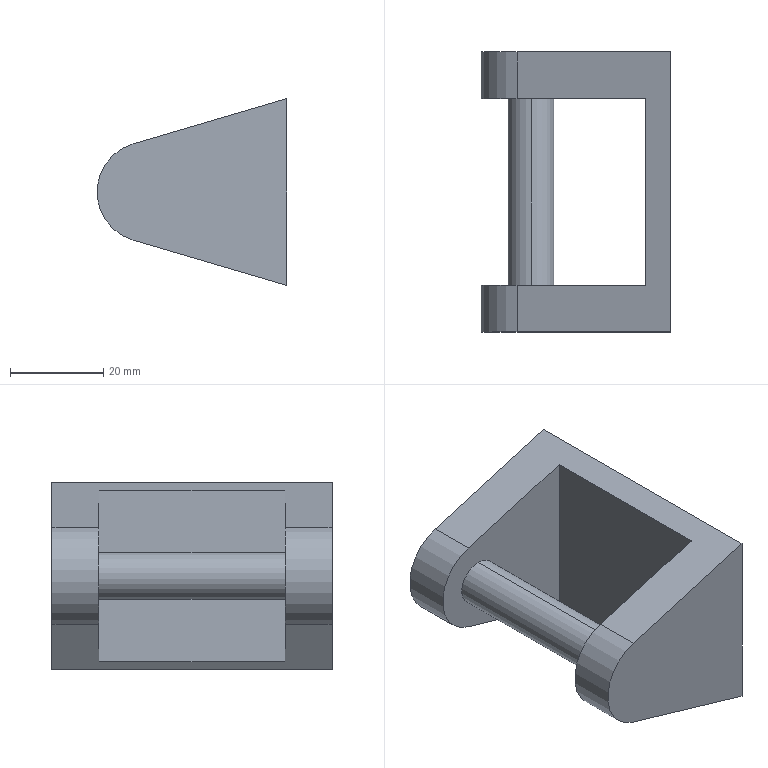Part | SolidWorks | features ICE 2, Extrusion 1 | 1 solid | 12 faces | box 40.645 x 60 x 40 mm | volume 33727 mm3 | plane 8 | cylinder 4 | commonest cylinder face diameters 10 x2 21.526 x2
STEP:
#1=CARTESIAN_POINT('',(-29.882,50.,15.));
#2=VERTEX_POINT('',#1);
#3=CARTESIAN_POINT('',(-29.882,50.,25.));
#4=VERTEX_POINT('',#3);
#5=CARTESIAN_POINT('',(-29.882,50.,20.));
#6=DIRECTION('',(0.,-1.,0.));
#7=DIRECTION('',(0.,0.,-1.));
#8=AXIS2_PLACEMENT_3D('',#5,#6,#7);
#9=CIRCLE('',#8,5.);
#10=EDGE_CURVE('',#2,#4,#9,.T.);
#11=ORIENTED_EDGE('',*,*,#10,.T.);
#12=CARTESIAN_POINT('',(-29.882,10.,25.));
#13=VERTEX_POINT('',#12);
#14=CARTESIAN_POINT('',(-29.882,60.002,25.));
#15=DIRECTION('',(0.,-1.,0.));
#16=VECTOR('',#15,1000.);
#17=LINE('',#14,#16);
#18=EDGE_CURVE('',#4,#13,#17,.T.);
#19=ORIENTED_EDGE('',*,*,#18,.T.);
#20=CARTESIAN_POINT('',(-29.882,10.,15.));
#21=VERTEX_POINT('',#20);
#22=CARTESIAN_POINT('',(-29.882,10.,20.));
#23=DIRECTION('',(0.,-1.,0.));
#24=DIRECTION('',(0.,0.,-1.));
#25=AXIS2_PLACEMENT_3D('',#22,#23,#24);
#26=CIRCLE('',#25,5.);
#27=EDGE_CURVE('',#21,#13,#26,.T.);
#28=ORIENTED_EDGE('',*,*,#27,.F.);
#29=CARTESIAN_POINT('',(-29.882,60.002,15.));
#30=DIRECTION('',(0.,-1.,0.));
#31=VECTOR('',#30,1000.);
#32=LINE('',#29,#31);
#33=EDGE_CURVE('',#2,#21,#32,.T.);
#34=ORIENTED_EDGE('',*,*,#33,.F.);
#35=EDGE_LOOP('',(#11,#19,#28,#34));
#36=FACE_OUTER_BOUND('',#35,.T.);
#37=CARTESIAN_POINT('',(-29.882,60.002,20.));
#38=DIRECTION('',(0.,-1.,0.));
#39=DIRECTION('',(0.,0.,-1.));
#40=AXIS2_PLACEMENT_3D('',#37,#38,#39);
#41=CYLINDRICAL_SURFACE('',#40,5.);
#42=ADVANCED_FACE('',(#36),#41,.T.);
#43=CARTESIAN_POINT('',(-32.917,50.,9.673));
#44=VERTEX_POINT('',#43);
#45=CARTESIAN_POINT('',(-5.382,50.,1.581));
#46=VERTEX_POINT('',#45);
#47=CARTESIAN_POINT('',(-32.917,50.,9.673));
#48=DIRECTION('',(0.9594,0.,-0.282));
#49=VECTOR('',#48,1000.);
#50=LINE('',#47,#49);
#51=EDGE_CURVE('',#44,#46,#50,.T.);
#52=ORIENTED_EDGE('',*,*,#51,.F.);
#53=CARTESIAN_POINT('',(-32.917,60.,9.673));
#54=VERTEX_POINT('',#53);
#55=CARTESIAN_POINT('',(-32.917,60.,9.673));
#56=DIRECTION('',(0.,-1.,0.));
#57=VECTOR('',#56,1000.);
#58=LINE('',#55,#57);
#59=EDGE_CURVE('',#54,#44,#58,.T.);
#60=ORIENTED_EDGE('',*,*,#59,.F.);
#61=CARTESIAN_POINT('',(0.,60.,0.));
#62=VERTEX_POINT('',#61);
#63=CARTESIAN_POINT('',(0.,60.,0.));
#64=DIRECTION('',(-0.9594,0.,0.282));
#65=VECTOR('',#64,1000.);
#66=LINE('',#63,#65);
#67=EDGE_CURVE('',#62,#54,#66,.T.);
#68=ORIENTED_EDGE('',*,*,#67,.F.);
#69=CARTESIAN_POINT('',(0.,0.,0.));
#70=VERTEX_POINT('',#69);
#71=CARTESIAN_POINT('',(0.,60.,0.));
#72=DIRECTION('',(0.,-1.,0.));
#73=VECTOR('',#72,1000.);
#74=LINE('',#71,#73);
#75=EDGE_CURVE('',#62,#70,#74,.T.);
#76=ORIENTED_EDGE('',*,*,#75,.T.);
#77=CARTESIAN_POINT('',(-32.917,0.,9.673));
#78=VERTEX_POINT('',#77);
#79=CARTESIAN_POINT('',(0.,0.,0.));
#80=DIRECTION('',(-0.9594,0.,0.282));
#81=VECTOR('',#80,1000.);
#82=LINE('',#79,#81);
#83=EDGE_CURVE('',#70,#78,#82,.T.);
#84=ORIENTED_EDGE('',*,*,#83,.T.);
#85=CARTESIAN_POINT('',(-32.917,10.,9.673));
#86=VERTEX_POINT('',#85);
#87=CARTESIAN_POINT('',(-32.917,60.,9.673));
#88=DIRECTION('',(0.,-1.,0.));
#89=VECTOR('',#88,1000.);
#90=LINE('',#87,#89);
#91=EDGE_CURVE('',#86,#78,#90,.T.);
#92=ORIENTED_EDGE('',*,*,#91,.F.);
#93=CARTESIAN_POINT('',(-5.382,10.,1.581));
#94=VERTEX_POINT('',#93);
#95=CARTESIAN_POINT('',(-32.917,10.,9.673));
#96=DIRECTION('',(0.9594,0.,-0.282));
#97=VECTOR('',#96,1000.);
#98=LINE('',#95,#97);
#99=EDGE_CURVE('',#86,#94,#98,.T.);
#100=ORIENTED_EDGE('',*,*,#99,.T.);
#101=CARTESIAN_POINT('',(-5.382,50.,1.581));
#102=DIRECTION('',(0.,-1.,0.));
#103=VECTOR('',#102,1000.);
#104=LINE('',#101,#103);
#105=EDGE_CURVE('',#46,#94,#104,.T.);
#106=ORIENTED_EDGE('',*,*,#105,.F.);
#107=EDGE_LOOP('',(#52,#60,#68,#76,#84,#92,#100,#106));
#108=FACE_OUTER_BOUND('',#107,.T.);
#109=CARTESIAN_POINT('',(0.,60.,0.));
#110=DIRECTION('',(0.282,0.,0.9594));
#111=DIRECTION('',(0.9594,0.,-0.282));
#112=AXIS2_PLACEMENT_3D('',#109,#110,#111);
#113=PLANE('',#112);
#114=ADVANCED_FACE('',(#108),#113,.F.);
#115=CARTESIAN_POINT('',(-32.917,50.,30.327));
#116=VERTEX_POINT('',#115);
#117=CARTESIAN_POINT('',(-29.882,50.,20.));
#118=DIRECTION('',(0.,-1.,0.));
#119=DIRECTION('',(0.,0.,-1.));
#120=AXIS2_PLACEMENT_3D('',#117,#118,#119);
#121=CIRCLE('',#120,10.763);
#122=EDGE_CURVE('',#116,#44,#121,.T.);
#123=ORIENTED_EDGE('',*,*,#122,.F.);
#124=CARTESIAN_POINT('',(-32.917,60.,30.327));
#125=VERTEX_POINT('',#124);
#126=CARTESIAN_POINT('',(-32.917,60.,30.327));
#127=DIRECTION('',(0.,-1.,0.));
#128=VECTOR('',#127,1000.);
#129=LINE('',#126,#128);
#130=EDGE_CURVE('',#125,#116,#129,.T.);
#131=ORIENTED_EDGE('',*,*,#130,.F.);
#132=CARTESIAN_POINT('',(-29.882,60.,20.));
#133=DIRECTION('',(0.,1.,0.));
#134=DIRECTION('',(0.,0.,-1.));
#135=AXIS2_PLACEMENT_3D('',#132,#133,#134);
#136=CIRCLE('',#135,10.763);
#137=EDGE_CURVE('',#54,#125,#136,.T.);
#138=ORIENTED_EDGE('',*,*,#137,.F.);
#139=ORIENTED_EDGE('',*,*,#59,.T.);
#140=EDGE_LOOP('',(#123,#131,#138,#139));
#141=FACE_OUTER_BOUND('',#140,.T.);
#142=CARTESIAN_POINT('',(-29.882,60.,20.));
#143=DIRECTION('',(0.,-1.,0.));
#144=DIRECTION('',(0.,0.,-1.));
#145=AXIS2_PLACEMENT_3D('',#142,#143,#144);
#146=CYLINDRICAL_SURFACE('',#145,10.763);
#147=ADVANCED_FACE('',(#141),#146,.T.);
#148=CARTESIAN_POINT('',(-5.382,50.,38.419));
#149=VERTEX_POINT('',#148);
#150=CARTESIAN_POINT('',(-5.382,50.,38.419));
#151=DIRECTION('',(-0.9594,0.,-0.282));
#152=VECTOR('',#151,1000.);
#153=LINE('',#150,#152);
#154=EDGE_CURVE('',#149,#116,#153,.T.);
#155=ORIENTED_EDGE('',*,*,#154,.F.);
#156=CARTESIAN_POINT('',(-5.382,10.,38.419));
#157=VERTEX_POINT('',#156);
#158=CARTESIAN_POINT('',(-5.382,50.,38.419));
#159=DIRECTION('',(0.,-1.,0.));
#160=VECTOR('',#159,1000.);
#161=LINE('',#158,#160);
#162=EDGE_CURVE('',#149,#157,#161,.T.);
#163=ORIENTED_EDGE('',*,*,#162,.T.);
#164=CARTESIAN_POINT('',(-32.917,10.,30.327));
#165=VERTEX_POINT('',#164);
#166=CARTESIAN_POINT('',(-5.382,10.,38.419));
#167=DIRECTION('',(-0.9594,0.,-0.282));
#168=VECTOR('',#167,1000.);
#169=LINE('',#166,#168);
#170=EDGE_CURVE('',#157,#165,#169,.T.);
#171=ORIENTED_EDGE('',*,*,#170,.T.);
#172=CARTESIAN_POINT('',(-32.917,0.,30.327));
#173=VERTEX_POINT('',#172);
#174=CARTESIAN_POINT('',(-32.917,60.,30.327));
#175=DIRECTION('',(0.,-1.,0.));
#176=VECTOR('',#175,1000.);
#177=LINE('',#174,#176);
#178=EDGE_CURVE('',#165,#173,#177,.T.);
#179=ORIENTED_EDGE('',*,*,#178,.T.);
#180=CARTESIAN_POINT('',(0.,0.,40.));
#181=VERTEX_POINT('',#180);
#182=CARTESIAN_POINT('',(0.,0.,40.));
#183=DIRECTION('',(0.9594,0.,0.282));
#184=VECTOR('',#183,1000.);
#185=LINE('',#182,#184);
#186=EDGE_CURVE('',#173,#181,#185,.T.);
#187=ORIENTED_EDGE('',*,*,#186,.T.);
#188=CARTESIAN_POINT('',(0.,60.,40.));
#189=VERTEX_POINT('',#188);
#190=CARTESIAN_POINT('',(0.,60.,40.));
#191=DIRECTION('',(0.,-1.,0.));
#192=VECTOR('',#191,1000.);
#193=LINE('',#190,#192);
#194=EDGE_CURVE('',#189,#181,#193,.T.);
#195=ORIENTED_EDGE('',*,*,#194,.F.);
#196=CARTESIAN_POINT('',(0.,60.,40.));
#197=DIRECTION('',(0.9594,0.,0.282));
#198=VECTOR('',#197,1000.);
#199=LINE('',#196,#198);
#200=EDGE_CURVE('',#125,#189,#199,.T.);
#201=ORIENTED_EDGE('',*,*,#200,.F.);
#202=ORIENTED_EDGE('',*,*,#130,.T.);
#203=EDGE_LOOP('',(#155,#163,#171,#179,#187,#195,#201,#202));
#204=FACE_OUTER_BOUND('',#203,.T.);
#205=CARTESIAN_POINT('',(0.,60.,40.));
#206=DIRECTION('',(0.282,0.,-0.9594));
#207=DIRECTION('',(-0.9594,0.,-0.282));
#208=AXIS2_PLACEMENT_3D('',#205,#206,#207);
#209=PLANE('',#208);
#210=ADVANCED_FACE('',(#204),#209,.F.);
#211=ORIENTED_EDGE('',*,*,#178,.F.);
#212=CARTESIAN_POINT('',(-29.882,10.,20.));
#213=DIRECTION('',(0.,-1.,0.));
#214=DIRECTION('',(0.,0.,-1.));
#215=AXIS2_PLACEMENT_3D('',#212,#213,#214);
#216=CIRCLE('',#215,10.763);
#217=EDGE_CURVE('',#165,#86,#216,.T.);
#218=ORIENTED_EDGE('',*,*,#217,.T.);
#219=ORIENTED_EDGE('',*,*,#91,.T.);
#220=CARTESIAN_POINT('',(-29.882,0.,20.));
#221=DIRECTION('',(0.,1.,0.));
#222=DIRECTION('',(0.,0.,-1.));
#223=AXIS2_PLACEMENT_3D('',#220,#221,#222);
#224=CIRCLE('',#223,10.763);
#225=EDGE_CURVE('',#78,#173,#224,.T.);
#226=ORIENTED_EDGE('',*,*,#225,.T.);
#227=EDGE_LOOP('',(#211,#218,#219,#226));
#228=FACE_OUTER_BOUND('',#227,.T.);
#229=CARTESIAN_POINT('',(-29.882,60.,20.));
#230=DIRECTION('',(0.,-1.,0.));
#231=DIRECTION('',(0.,0.,-1.));
#232=AXIS2_PLACEMENT_3D('',#229,#230,#231);
#233=CYLINDRICAL_SURFACE('',#232,10.763);
#234=ADVANCED_FACE('',(#228),#233,.T.);
#235=CARTESIAN_POINT('',(0.,0.,0.));
#236=DIRECTION('',(0.,0.,-1.));
#237=VECTOR('',#236,1000.);
#238=LINE('',#235,#237);
#239=EDGE_CURVE('',#181,#70,#238,.T.);
#240=ORIENTED_EDGE('',*,*,#239,.T.);
#241=ORIENTED_EDGE('',*,*,#75,.F.);
#242=CARTESIAN_POINT('',(0.,60.,0.));
#243=DIRECTION('',(0.,0.,-1.));
#244=VECTOR('',#243,1000.);
#245=LINE('',#242,#244);
#246=EDGE_CURVE('',#189,#62,#245,.T.);
#247=ORIENTED_EDGE('',*,*,#246,.F.);
#248=ORIENTED_EDGE('',*,*,#194,.T.);
#249=EDGE_LOOP('',(#240,#241,#247,#248));
#250=FACE_OUTER_BOUND('',#249,.T.);
#251=CARTESIAN_POINT('',(0.,60.,0.));
#252=DIRECTION('',(-1.,0.,0.));
#253=DIRECTION('',(0.,0.,1.));
#254=AXIS2_PLACEMENT_3D('',#251,#252,#253);
#255=PLANE('',#254);
#256=ADVANCED_FACE('',(#250),#255,.F.);
#257=ORIENTED_EDGE('',*,*,#67,.T.);
#258=ORIENTED_EDGE('',*,*,#137,.T.);
#259=ORIENTED_EDGE('',*,*,#200,.T.);
#260=ORIENTED_EDGE('',*,*,#246,.T.);
#261=EDGE_LOOP('',(#257,#258,#259,#260));
#262=FACE_OUTER_BOUND('',#261,.T.);
#263=CARTESIAN_POINT('',(-29.882,60.,20.));
#264=DIRECTION('',(0.,-1.,0.));
#265=DIRECTION('',(0.,0.,-1.));
#266=AXIS2_PLACEMENT_3D('',#263,#264,#265);
#267=PLANE('',#266);
#268=ADVANCED_FACE('',(#262),#267,.F.);
#269=ORIENTED_EDGE('',*,*,#83,.F.);
#270=ORIENTED_EDGE('',*,*,#239,.F.);
#271=ORIENTED_EDGE('',*,*,#186,.F.);
#272=ORIENTED_EDGE('',*,*,#225,.F.);
#273=EDGE_LOOP('',(#269,#270,#271,#272));
#274=FACE_OUTER_BOUND('',#273,.T.);
#275=CARTESIAN_POINT('',(-29.882,0.,20.));
#276=DIRECTION('',(0.,-1.,0.));
#277=DIRECTION('',(0.,0.,-1.));
#278=AXIS2_PLACEMENT_3D('',#275,#276,#277);
#279=PLANE('',#278);
#280=ADVANCED_FACE('',(#274),#279,.T.);
#281=CARTESIAN_POINT('',(-5.382,10.,1.581));
#282=DIRECTION('',(0.,0.,1.));
#283=VECTOR('',#282,1000.);
#284=LINE('',#281,#283);
#285=EDGE_CURVE('',#94,#157,#284,.T.);
#286=ORIENTED_EDGE('',*,*,#285,.T.);
#287=ORIENTED_EDGE('',*,*,#162,.F.);
#288=CARTESIAN_POINT('',(-5.382,50.,1.581));
#289=DIRECTION('',(0.,0.,1.));
#290=VECTOR('',#289,1000.);
#291=LINE('',#288,#290);
#292=EDGE_CURVE('',#46,#149,#291,.T.);
#293=ORIENTED_EDGE('',*,*,#292,.F.);
#294=ORIENTED_EDGE('',*,*,#105,.T.);
#295=EDGE_LOOP('',(#286,#287,#293,#294));
#296=FACE_OUTER_BOUND('',#295,.T.);
#297=CARTESIAN_POINT('',(-5.382,50.,1.581));
#298=DIRECTION('',(1.,0.,0.));
#299=DIRECTION('',(0.,0.,-1.));
#300=AXIS2_PLACEMENT_3D('',#297,#298,#299);
#301=PLANE('',#300);
#302=ADVANCED_FACE('',(#296),#301,.F.);
#303=ORIENTED_EDGE('',*,*,#10,.F.);
#304=CARTESIAN_POINT('',(-29.882,50.,20.));
#305=DIRECTION('',(0.,-1.,0.));
#306=DIRECTION('',(0.,0.,-1.));
#307=AXIS2_PLACEMENT_3D('',#304,#305,#306);
#308=CIRCLE('',#307,5.);
#309=EDGE_CURVE('',#4,#2,#308,.T.);
#310=ORIENTED_EDGE('',*,*,#309,.F.);
#311=EDGE_LOOP('',(#303,#310));
#312=FACE_BOUND('',#311,.T.);
#313=ORIENTED_EDGE('',*,*,#51,.T.);
#314=ORIENTED_EDGE('',*,*,#292,.T.);
#315=ORIENTED_EDGE('',*,*,#154,.T.);
#316=ORIENTED_EDGE('',*,*,#122,.T.);
#317=EDGE_LOOP('',(#313,#314,#315,#316));
#318=FACE_OUTER_BOUND('',#317,.T.);
#319=CARTESIAN_POINT('',(-29.882,50.,20.));
#320=DIRECTION('',(0.,-1.,0.));
#321=DIRECTION('',(0.,0.,-1.));
#322=AXIS2_PLACEMENT_3D('',#319,#320,#321);
#323=PLANE('',#322);
#324=ADVANCED_FACE('',(#312,#318),#323,.T.);
#325=ORIENTED_EDGE('',*,*,#27,.T.);
#326=CARTESIAN_POINT('',(-29.882,10.,20.));
#327=DIRECTION('',(0.,-1.,0.));
#328=DIRECTION('',(0.,0.,-1.));
#329=AXIS2_PLACEMENT_3D('',#326,#327,#328);
#330=CIRCLE('',#329,5.);
#331=EDGE_CURVE('',#13,#21,#330,.T.);
#332=ORIENTED_EDGE('',*,*,#331,.T.);
#333=EDGE_LOOP('',(#325,#332));
#334=FACE_BOUND('',#333,.T.);
#335=ORIENTED_EDGE('',*,*,#99,.F.);
#336=ORIENTED_EDGE('',*,*,#217,.F.);
#337=ORIENTED_EDGE('',*,*,#170,.F.);
#338=ORIENTED_EDGE('',*,*,#285,.F.);
#339=EDGE_LOOP('',(#335,#336,#337,#338));
#340=FACE_OUTER_BOUND('',#339,.T.);
#341=CARTESIAN_POINT('',(-29.882,10.,20.));
#342=DIRECTION('',(0.,-1.,0.));
#343=DIRECTION('',(0.,0.,-1.));
#344=AXIS2_PLACEMENT_3D('',#341,#342,#343);
#345=PLANE('',#344);
#346=ADVANCED_FACE('',(#334,#340),#345,.F.);
#347=ORIENTED_EDGE('',*,*,#18,.F.);
#348=ORIENTED_EDGE('',*,*,#309,.T.);
#349=ORIENTED_EDGE('',*,*,#33,.T.);
#350=ORIENTED_EDGE('',*,*,#331,.F.);
#351=EDGE_LOOP('',(#347,#348,#349,#350));
#352=FACE_OUTER_BOUND('',#351,.T.);
#353=CARTESIAN_POINT('',(-29.882,60.002,20.));
#354=DIRECTION('',(0.,-1.,0.));
#355=DIRECTION('',(0.,0.,-1.));
#356=AXIS2_PLACEMENT_3D('',#353,#354,#355);
#357=CYLINDRICAL_SURFACE('',#356,5.);
#358=ADVANCED_FACE('',(#352),#357,.T.);
#359=CLOSED_SHELL('',(#42,#114,#147,#210,#234,#256,#268,#280,#302,#324,#346,#358));
#360=MANIFOLD_SOLID_BREP('',#359);
#361=CARTESIAN_POINT('',(0.,0.,0.));
#362=DIRECTION('',(0.,0.,1.));
#363=DIRECTION('',(1.,0.,0.));
#364=AXIS2_PLACEMENT_3D('',#361,#362,#363);
#365=(LENGTH_UNIT()NAMED_UNIT(*)SI_UNIT(.MILLI.,.METRE.));
#366=UNCERTAINTY_MEASURE_WITH_UNIT(LENGTH_MEASURE(0.00001),#365,'','');
#367=(NAMED_UNIT(*)PLANE_ANGLE_UNIT()SI_UNIT($,.RADIAN.));
#368=(NAMED_UNIT(*)SI_UNIT($,.STERADIAN.)SOLID_ANGLE_UNIT());
#369=(GEOMETRIC_REPRESENTATION_CONTEXT(3)GLOBAL_UNCERTAINTY_ASSIGNED_CONTEXT((#366))GLOBAL_UNIT_ASSIGNED_CONTEXT((#365,#367,#368))REPRESENTATION_CONTEXT('',''));
#370=ADVANCED_BREP_SHAPE_REPRESENTATION('',(#360,#364),#369);